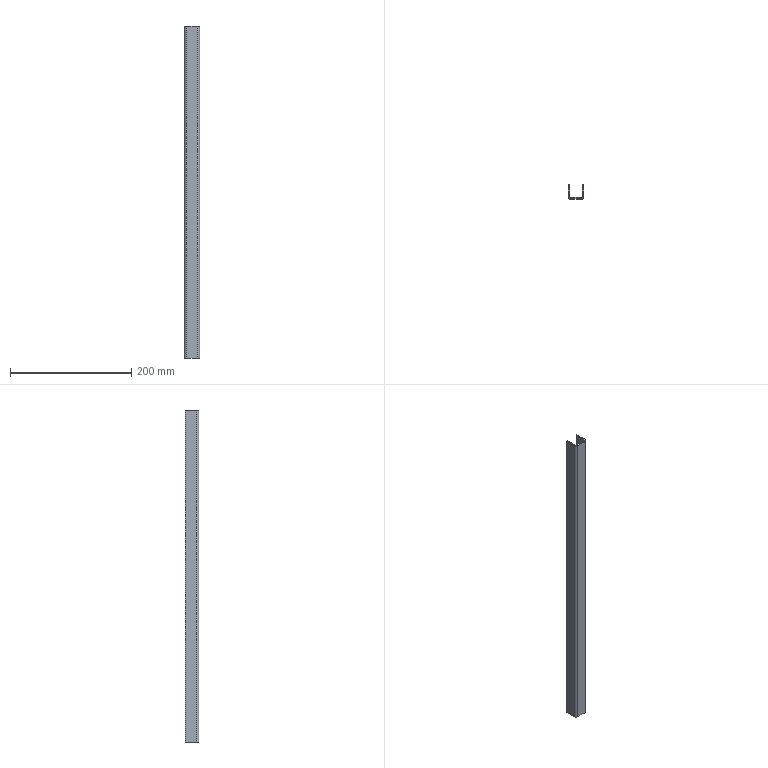Part | NX | features solid 2 | 1 solid | 14 faces | box 25 x 23 x 547 mm | volume 70481 mm3 | plane 10 | cylinder 4 | commonest cylinder face diameters 4 x2 8 x2
STEP:
#1=CARTESIAN_POINT('',(1215.,-671.,1137.));
#2=VERTEX_POINT('',#1);
#3=CARTESIAN_POINT('',(1215.,-652.,1137.));
#4=VERTEX_POINT('',#3);
#5=CARTESIAN_POINT('',(1215.,-652.,1137.));
#6=DIRECTION('',(0.,1.,0.));
#7=VECTOR('',#6,1000.);
#8=LINE('',#5,#7);
#9=EDGE_CURVE('',#2,#4,#8,.T.);
#10=ORIENTED_EDGE('',*,*,#9,.T.);
#11=CARTESIAN_POINT('',(1215.,-652.,590.));
#12=VERTEX_POINT('',#11);
#13=CARTESIAN_POINT('',(1215.,-652.,590.));
#14=DIRECTION('',(0.,0.,1.));
#15=VECTOR('',#14,1000.);
#16=LINE('',#13,#15);
#17=EDGE_CURVE('',#12,#4,#16,.T.);
#18=ORIENTED_EDGE('',*,*,#17,.F.);
#19=CARTESIAN_POINT('',(1215.,-671.,590.));
#20=VERTEX_POINT('',#19);
#21=CARTESIAN_POINT('',(1215.,-652.,590.));
#22=DIRECTION('',(0.,1.,0.));
#23=VECTOR('',#22,1000.);
#24=LINE('',#21,#23);
#25=EDGE_CURVE('',#20,#12,#24,.T.);
#26=ORIENTED_EDGE('',*,*,#25,.F.);
#27=CARTESIAN_POINT('',(1215.,-671.,590.));
#28=DIRECTION('',(0.,0.,1.));
#29=VECTOR('',#28,1000.);
#30=LINE('',#27,#29);
#31=EDGE_CURVE('',#20,#2,#30,.T.);
#32=ORIENTED_EDGE('',*,*,#31,.T.);
#33=EDGE_LOOP('',(#10,#18,#26,#32));
#34=FACE_BOUND('',#33,.T.);
#35=CARTESIAN_POINT('',(1215.,-652.,590.));
#36=DIRECTION('',(1.,0.,0.));
#37=DIRECTION('',(0.,0.,1.));
#38=AXIS2_PLACEMENT_3D('',#35,#36,#37);
#39=PLANE('',#38);
#40=ADVANCED_FACE('',(#34),#39,.F.);
#41=CARTESIAN_POINT('',(1219.,-675.,1137.));
#42=VERTEX_POINT('',#41);
#43=CARTESIAN_POINT('',(1219.,-671.,1137.));
#44=DIRECTION('',(0.,0.,-1.));
#45=DIRECTION('',(0.,-1.,0.));
#46=AXIS2_PLACEMENT_3D('',#43,#44,#45);
#47=CIRCLE('',#46,4.);
#48=EDGE_CURVE('',#42,#2,#47,.T.);
#49=ORIENTED_EDGE('',*,*,#48,.T.);
#50=ORIENTED_EDGE('',*,*,#31,.F.);
#51=CARTESIAN_POINT('',(1219.,-675.,590.));
#52=VERTEX_POINT('',#51);
#53=CARTESIAN_POINT('',(1219.,-671.,590.));
#54=DIRECTION('',(0.,0.,-1.));
#55=DIRECTION('',(0.,-1.,0.));
#56=AXIS2_PLACEMENT_3D('',#53,#54,#55);
#57=CIRCLE('',#56,4.);
#58=EDGE_CURVE('',#52,#20,#57,.T.);
#59=ORIENTED_EDGE('',*,*,#58,.F.);
#60=CARTESIAN_POINT('',(1219.,-675.,590.));
#61=DIRECTION('',(0.,0.,1.));
#62=VECTOR('',#61,1000.);
#63=LINE('',#60,#62);
#64=EDGE_CURVE('',#52,#42,#63,.T.);
#65=ORIENTED_EDGE('',*,*,#64,.T.);
#66=EDGE_LOOP('',(#49,#50,#59,#65));
#67=FACE_BOUND('',#66,.T.);
#68=CARTESIAN_POINT('',(1219.,-671.,590.));
#69=DIRECTION('',(0.,0.,1.));
#70=DIRECTION('',(0.,-1.,0.));
#71=AXIS2_PLACEMENT_3D('',#68,#69,#70);
#72=CYLINDRICAL_SURFACE('',#71,4.);
#73=ADVANCED_FACE('',(#67),#72,.T.);
#74=CARTESIAN_POINT('',(1236.,-675.,1137.));
#75=VERTEX_POINT('',#74);
#76=CARTESIAN_POINT('',(1217.,-675.,1137.));
#77=DIRECTION('',(-1.,0.,0.));
#78=VECTOR('',#77,1000.);
#79=LINE('',#76,#78);
#80=EDGE_CURVE('',#75,#42,#79,.T.);
#81=ORIENTED_EDGE('',*,*,#80,.T.);
#82=ORIENTED_EDGE('',*,*,#64,.F.);
#83=CARTESIAN_POINT('',(1236.,-675.,590.));
#84=VERTEX_POINT('',#83);
#85=CARTESIAN_POINT('',(1217.,-675.,590.));
#86=DIRECTION('',(-1.,0.,0.));
#87=VECTOR('',#86,1000.);
#88=LINE('',#85,#87);
#89=EDGE_CURVE('',#84,#52,#88,.T.);
#90=ORIENTED_EDGE('',*,*,#89,.F.);
#91=CARTESIAN_POINT('',(1236.,-675.,590.));
#92=DIRECTION('',(0.,0.,1.));
#93=VECTOR('',#92,1000.);
#94=LINE('',#91,#93);
#95=EDGE_CURVE('',#84,#75,#94,.T.);
#96=ORIENTED_EDGE('',*,*,#95,.T.);
#97=EDGE_LOOP('',(#81,#82,#90,#96));
#98=FACE_BOUND('',#97,.T.);
#99=CARTESIAN_POINT('',(1217.,-675.,590.));
#100=DIRECTION('',(0.,1.,0.));
#101=DIRECTION('',(0.,0.,-1.));
#102=AXIS2_PLACEMENT_3D('',#99,#100,#101);
#103=PLANE('',#102);
#104=ADVANCED_FACE('',(#98),#103,.F.);
#105=CARTESIAN_POINT('',(1240.,-671.,1137.));
#106=VERTEX_POINT('',#105);
#107=CARTESIAN_POINT('',(1236.,-671.,1137.));
#108=DIRECTION('',(0.,0.,-1.));
#109=DIRECTION('',(0.,-1.,0.));
#110=AXIS2_PLACEMENT_3D('',#107,#108,#109);
#111=CIRCLE('',#110,4.);
#112=EDGE_CURVE('',#106,#75,#111,.T.);
#113=ORIENTED_EDGE('',*,*,#112,.T.);
#114=ORIENTED_EDGE('',*,*,#95,.F.);
#115=CARTESIAN_POINT('',(1240.,-671.,590.));
#116=VERTEX_POINT('',#115);
#117=CARTESIAN_POINT('',(1236.,-671.,590.));
#118=DIRECTION('',(0.,0.,-1.));
#119=DIRECTION('',(0.,-1.,0.));
#120=AXIS2_PLACEMENT_3D('',#117,#118,#119);
#121=CIRCLE('',#120,4.);
#122=EDGE_CURVE('',#116,#84,#121,.T.);
#123=ORIENTED_EDGE('',*,*,#122,.F.);
#124=CARTESIAN_POINT('',(1240.,-671.,590.));
#125=DIRECTION('',(0.,0.,1.));
#126=VECTOR('',#125,1000.);
#127=LINE('',#124,#126);
#128=EDGE_CURVE('',#116,#106,#127,.T.);
#129=ORIENTED_EDGE('',*,*,#128,.T.);
#130=EDGE_LOOP('',(#113,#114,#123,#129));
#131=FACE_BOUND('',#130,.T.);
#132=CARTESIAN_POINT('',(1236.,-671.,590.));
#133=DIRECTION('',(0.,0.,1.));
#134=DIRECTION('',(0.,-1.,0.));
#135=AXIS2_PLACEMENT_3D('',#132,#133,#134);
#136=CYLINDRICAL_SURFACE('',#135,4.);
#137=ADVANCED_FACE('',(#131),#136,.T.);
#138=CARTESIAN_POINT('',(1240.,-652.,1137.));
#139=VERTEX_POINT('',#138);
#140=CARTESIAN_POINT('',(1240.,-673.,1137.));
#141=DIRECTION('',(0.,-1.,0.));
#142=VECTOR('',#141,1000.);
#143=LINE('',#140,#142);
#144=EDGE_CURVE('',#139,#106,#143,.T.);
#145=ORIENTED_EDGE('',*,*,#144,.T.);
#146=ORIENTED_EDGE('',*,*,#128,.F.);
#147=CARTESIAN_POINT('',(1240.,-652.,590.));
#148=VERTEX_POINT('',#147);
#149=CARTESIAN_POINT('',(1240.,-673.,590.));
#150=DIRECTION('',(0.,-1.,0.));
#151=VECTOR('',#150,1000.);
#152=LINE('',#149,#151);
#153=EDGE_CURVE('',#148,#116,#152,.T.);
#154=ORIENTED_EDGE('',*,*,#153,.F.);
#155=CARTESIAN_POINT('',(1240.,-652.,590.));
#156=DIRECTION('',(0.,0.,1.));
#157=VECTOR('',#156,1000.);
#158=LINE('',#155,#157);
#159=EDGE_CURVE('',#148,#139,#158,.T.);
#160=ORIENTED_EDGE('',*,*,#159,.T.);
#161=EDGE_LOOP('',(#145,#146,#154,#160));
#162=FACE_BOUND('',#161,.T.);
#163=CARTESIAN_POINT('',(1240.,-673.,590.));
#164=DIRECTION('',(-1.,0.,0.));
#165=DIRECTION('',(0.,0.,1.));
#166=AXIS2_PLACEMENT_3D('',#163,#164,#165);
#167=PLANE('',#166);
#168=ADVANCED_FACE('',(#162),#167,.F.);
#169=CARTESIAN_POINT('',(1217.,-671.,1137.));
#170=VERTEX_POINT('',#169);
#171=CARTESIAN_POINT('',(1217.,-652.,1137.));
#172=VERTEX_POINT('',#171);
#173=CARTESIAN_POINT('',(1217.,-652.,1137.));
#174=DIRECTION('',(0.,1.,0.));
#175=VECTOR('',#174,1000.);
#176=LINE('',#173,#175);
#177=EDGE_CURVE('',#170,#172,#176,.T.);
#178=ORIENTED_EDGE('',*,*,#177,.F.);
#179=CARTESIAN_POINT('',(1217.,-671.,590.));
#180=VERTEX_POINT('',#179);
#181=CARTESIAN_POINT('',(1217.,-671.,590.));
#182=DIRECTION('',(0.,0.,1.));
#183=VECTOR('',#182,1000.);
#184=LINE('',#181,#183);
#185=EDGE_CURVE('',#180,#170,#184,.T.);
#186=ORIENTED_EDGE('',*,*,#185,.F.);
#187=CARTESIAN_POINT('',(1217.,-652.,590.));
#188=VERTEX_POINT('',#187);
#189=CARTESIAN_POINT('',(1217.,-652.,590.));
#190=DIRECTION('',(0.,1.,0.));
#191=VECTOR('',#190,1000.);
#192=LINE('',#189,#191);
#193=EDGE_CURVE('',#180,#188,#192,.T.);
#194=ORIENTED_EDGE('',*,*,#193,.T.);
#195=CARTESIAN_POINT('',(1217.,-652.,590.));
#196=DIRECTION('',(0.,0.,1.));
#197=VECTOR('',#196,1000.);
#198=LINE('',#195,#197);
#199=EDGE_CURVE('',#188,#172,#198,.T.);
#200=ORIENTED_EDGE('',*,*,#199,.T.);
#201=EDGE_LOOP('',(#178,#186,#194,#200));
#202=FACE_BOUND('',#201,.T.);
#203=CARTESIAN_POINT('',(1217.,-652.,590.));
#204=DIRECTION('',(1.,0.,0.));
#205=DIRECTION('',(0.,0.,1.));
#206=AXIS2_PLACEMENT_3D('',#203,#204,#205);
#207=PLANE('',#206);
#208=ADVANCED_FACE('',(#202),#207,.T.);
#209=CARTESIAN_POINT('',(1219.,-673.,1137.));
#210=VERTEX_POINT('',#209);
#211=CARTESIAN_POINT('',(1219.,-671.,1137.));
#212=DIRECTION('',(0.,0.,-1.));
#213=DIRECTION('',(0.,-1.,0.));
#214=AXIS2_PLACEMENT_3D('',#211,#212,#213);
#215=CIRCLE('',#214,2.);
#216=EDGE_CURVE('',#210,#170,#215,.T.);
#217=ORIENTED_EDGE('',*,*,#216,.F.);
#218=CARTESIAN_POINT('',(1219.,-673.,590.));
#219=VERTEX_POINT('',#218);
#220=CARTESIAN_POINT('',(1219.,-673.,590.));
#221=DIRECTION('',(0.,0.,1.));
#222=VECTOR('',#221,1000.);
#223=LINE('',#220,#222);
#224=EDGE_CURVE('',#219,#210,#223,.T.);
#225=ORIENTED_EDGE('',*,*,#224,.F.);
#226=CARTESIAN_POINT('',(1219.,-671.,590.));
#227=DIRECTION('',(0.,0.,-1.));
#228=DIRECTION('',(0.,-1.,0.));
#229=AXIS2_PLACEMENT_3D('',#226,#227,#228);
#230=CIRCLE('',#229,2.);
#231=EDGE_CURVE('',#219,#180,#230,.T.);
#232=ORIENTED_EDGE('',*,*,#231,.T.);
#233=ORIENTED_EDGE('',*,*,#185,.T.);
#234=EDGE_LOOP('',(#217,#225,#232,#233));
#235=FACE_BOUND('',#234,.T.);
#236=CARTESIAN_POINT('',(1219.,-671.,590.));
#237=DIRECTION('',(0.,0.,1.));
#238=DIRECTION('',(0.,-1.,0.));
#239=AXIS2_PLACEMENT_3D('',#236,#237,#238);
#240=CYLINDRICAL_SURFACE('',#239,2.);
#241=ADVANCED_FACE('',(#235),#240,.F.);
#242=CARTESIAN_POINT('',(1236.,-673.,1137.));
#243=VERTEX_POINT('',#242);
#244=CARTESIAN_POINT('',(1217.,-673.,1137.));
#245=DIRECTION('',(-1.,0.,0.));
#246=VECTOR('',#245,1000.);
#247=LINE('',#244,#246);
#248=EDGE_CURVE('',#243,#210,#247,.T.);
#249=ORIENTED_EDGE('',*,*,#248,.F.);
#250=CARTESIAN_POINT('',(1236.,-673.,590.));
#251=VERTEX_POINT('',#250);
#252=CARTESIAN_POINT('',(1236.,-673.,590.));
#253=DIRECTION('',(0.,0.,1.));
#254=VECTOR('',#253,1000.);
#255=LINE('',#252,#254);
#256=EDGE_CURVE('',#251,#243,#255,.T.);
#257=ORIENTED_EDGE('',*,*,#256,.F.);
#258=CARTESIAN_POINT('',(1217.,-673.,590.));
#259=DIRECTION('',(-1.,0.,0.));
#260=VECTOR('',#259,1000.);
#261=LINE('',#258,#260);
#262=EDGE_CURVE('',#251,#219,#261,.T.);
#263=ORIENTED_EDGE('',*,*,#262,.T.);
#264=ORIENTED_EDGE('',*,*,#224,.T.);
#265=EDGE_LOOP('',(#249,#257,#263,#264));
#266=FACE_BOUND('',#265,.T.);
#267=CARTESIAN_POINT('',(1217.,-673.,590.));
#268=DIRECTION('',(0.,1.,0.));
#269=DIRECTION('',(0.,0.,-1.));
#270=AXIS2_PLACEMENT_3D('',#267,#268,#269);
#271=PLANE('',#270);
#272=ADVANCED_FACE('',(#266),#271,.T.);
#273=CARTESIAN_POINT('',(1238.,-671.,1137.));
#274=VERTEX_POINT('',#273);
#275=CARTESIAN_POINT('',(1236.,-671.,1137.));
#276=DIRECTION('',(0.,0.,-1.));
#277=DIRECTION('',(0.,-1.,0.));
#278=AXIS2_PLACEMENT_3D('',#275,#276,#277);
#279=CIRCLE('',#278,2.);
#280=EDGE_CURVE('',#274,#243,#279,.T.);
#281=ORIENTED_EDGE('',*,*,#280,.F.);
#282=CARTESIAN_POINT('',(1238.,-671.,590.));
#283=VERTEX_POINT('',#282);
#284=CARTESIAN_POINT('',(1238.,-671.,590.));
#285=DIRECTION('',(0.,0.,1.));
#286=VECTOR('',#285,1000.);
#287=LINE('',#284,#286);
#288=EDGE_CURVE('',#283,#274,#287,.T.);
#289=ORIENTED_EDGE('',*,*,#288,.F.);
#290=CARTESIAN_POINT('',(1236.,-671.,590.));
#291=DIRECTION('',(0.,0.,-1.));
#292=DIRECTION('',(0.,-1.,0.));
#293=AXIS2_PLACEMENT_3D('',#290,#291,#292);
#294=CIRCLE('',#293,2.);
#295=EDGE_CURVE('',#283,#251,#294,.T.);
#296=ORIENTED_EDGE('',*,*,#295,.T.);
#297=ORIENTED_EDGE('',*,*,#256,.T.);
#298=EDGE_LOOP('',(#281,#289,#296,#297));
#299=FACE_BOUND('',#298,.T.);
#300=CARTESIAN_POINT('',(1236.,-671.,590.));
#301=DIRECTION('',(0.,0.,1.));
#302=DIRECTION('',(0.,-1.,0.));
#303=AXIS2_PLACEMENT_3D('',#300,#301,#302);
#304=CYLINDRICAL_SURFACE('',#303,2.);
#305=ADVANCED_FACE('',(#299),#304,.F.);
#306=CARTESIAN_POINT('',(1238.,-652.,1137.));
#307=VERTEX_POINT('',#306);
#308=CARTESIAN_POINT('',(1238.,-673.,1137.));
#309=DIRECTION('',(0.,-1.,0.));
#310=VECTOR('',#309,1000.);
#311=LINE('',#308,#310);
#312=EDGE_CURVE('',#307,#274,#311,.T.);
#313=ORIENTED_EDGE('',*,*,#312,.F.);
#314=CARTESIAN_POINT('',(1238.,-652.,590.));
#315=VERTEX_POINT('',#314);
#316=CARTESIAN_POINT('',(1238.,-652.,590.));
#317=DIRECTION('',(0.,0.,1.));
#318=VECTOR('',#317,1000.);
#319=LINE('',#316,#318);
#320=EDGE_CURVE('',#315,#307,#319,.T.);
#321=ORIENTED_EDGE('',*,*,#320,.F.);
#322=CARTESIAN_POINT('',(1238.,-673.,590.));
#323=DIRECTION('',(0.,-1.,0.));
#324=VECTOR('',#323,1000.);
#325=LINE('',#322,#324);
#326=EDGE_CURVE('',#315,#283,#325,.T.);
#327=ORIENTED_EDGE('',*,*,#326,.T.);
#328=ORIENTED_EDGE('',*,*,#288,.T.);
#329=EDGE_LOOP('',(#313,#321,#327,#328));
#330=FACE_BOUND('',#329,.T.);
#331=CARTESIAN_POINT('',(1238.,-673.,590.));
#332=DIRECTION('',(-1.,0.,0.));
#333=DIRECTION('',(0.,0.,1.));
#334=AXIS2_PLACEMENT_3D('',#331,#332,#333);
#335=PLANE('',#334);
#336=ADVANCED_FACE('',(#330),#335,.T.);
#337=ORIENTED_EDGE('',*,*,#159,.F.);
#338=CARTESIAN_POINT('',(1238.,-652.,590.));
#339=DIRECTION('',(-1.,0.,0.));
#340=VECTOR('',#339,1000.);
#341=LINE('',#338,#340);
#342=EDGE_CURVE('',#148,#315,#341,.T.);
#343=ORIENTED_EDGE('',*,*,#342,.T.);
#344=ORIENTED_EDGE('',*,*,#320,.T.);
#345=CARTESIAN_POINT('',(1238.,-652.,1137.));
#346=DIRECTION('',(-1.,0.,0.));
#347=VECTOR('',#346,1000.);
#348=LINE('',#345,#347);
#349=EDGE_CURVE('',#139,#307,#348,.T.);
#350=ORIENTED_EDGE('',*,*,#349,.F.);
#351=EDGE_LOOP('',(#337,#343,#344,#350));
#352=FACE_BOUND('',#351,.T.);
#353=CARTESIAN_POINT('',(1238.,-652.,590.));
#354=DIRECTION('',(0.,-1.,0.));
#355=DIRECTION('',(-1.,0.,0.));
#356=AXIS2_PLACEMENT_3D('',#353,#354,#355);
#357=PLANE('',#356);
#358=ADVANCED_FACE('',(#352),#357,.F.);
#359=ORIENTED_EDGE('',*,*,#312,.T.);
#360=ORIENTED_EDGE('',*,*,#280,.T.);
#361=ORIENTED_EDGE('',*,*,#248,.T.);
#362=ORIENTED_EDGE('',*,*,#216,.T.);
#363=ORIENTED_EDGE('',*,*,#177,.T.);
#364=CARTESIAN_POINT('',(1217.,-652.,1137.));
#365=DIRECTION('',(1.,0.,0.));
#366=VECTOR('',#365,1000.);
#367=LINE('',#364,#366);
#368=EDGE_CURVE('',#4,#172,#367,.T.);
#369=ORIENTED_EDGE('',*,*,#368,.F.);
#370=ORIENTED_EDGE('',*,*,#9,.F.);
#371=ORIENTED_EDGE('',*,*,#48,.F.);
#372=ORIENTED_EDGE('',*,*,#80,.F.);
#373=ORIENTED_EDGE('',*,*,#112,.F.);
#374=ORIENTED_EDGE('',*,*,#144,.F.);
#375=ORIENTED_EDGE('',*,*,#349,.T.);
#376=EDGE_LOOP('',(#359,#360,#361,#362,#363,#369,#370,#371,#372,#373,#374,#375));
#377=FACE_BOUND('',#376,.T.);
#378=CARTESIAN_POINT('',(1238.,-673.,1137.));
#379=DIRECTION('',(0.,0.,-1.));
#380=DIRECTION('',(0.,-1.,0.));
#381=AXIS2_PLACEMENT_3D('',#378,#379,#380);
#382=PLANE('',#381);
#383=ADVANCED_FACE('',(#377),#382,.F.);
#384=CARTESIAN_POINT('',(1217.,-652.,590.));
#385=DIRECTION('',(1.,0.,0.));
#386=VECTOR('',#385,1000.);
#387=LINE('',#384,#386);
#388=EDGE_CURVE('',#12,#188,#387,.T.);
#389=ORIENTED_EDGE('',*,*,#388,.F.);
#390=ORIENTED_EDGE('',*,*,#17,.T.);
#391=ORIENTED_EDGE('',*,*,#368,.T.);
#392=ORIENTED_EDGE('',*,*,#199,.F.);
#393=EDGE_LOOP('',(#389,#390,#391,#392));
#394=FACE_BOUND('',#393,.T.);
#395=CARTESIAN_POINT('',(1217.,-652.,590.));
#396=DIRECTION('',(0.,1.,0.));
#397=DIRECTION('',(0.,0.,-1.));
#398=AXIS2_PLACEMENT_3D('',#395,#396,#397);
#399=PLANE('',#398);
#400=ADVANCED_FACE('',(#394),#399,.T.);
#401=ORIENTED_EDGE('',*,*,#193,.F.);
#402=ORIENTED_EDGE('',*,*,#231,.F.);
#403=ORIENTED_EDGE('',*,*,#262,.F.);
#404=ORIENTED_EDGE('',*,*,#295,.F.);
#405=ORIENTED_EDGE('',*,*,#326,.F.);
#406=ORIENTED_EDGE('',*,*,#342,.F.);
#407=ORIENTED_EDGE('',*,*,#153,.T.);
#408=ORIENTED_EDGE('',*,*,#122,.T.);
#409=ORIENTED_EDGE('',*,*,#89,.T.);
#410=ORIENTED_EDGE('',*,*,#58,.T.);
#411=ORIENTED_EDGE('',*,*,#25,.T.);
#412=ORIENTED_EDGE('',*,*,#388,.T.);
#413=EDGE_LOOP('',(#401,#402,#403,#404,#405,#406,#407,#408,#409,#410,#411,#412));
#414=FACE_BOUND('',#413,.T.);
#415=CARTESIAN_POINT('',(1217.,-652.,590.));
#416=DIRECTION('',(0.,0.,-1.));
#417=DIRECTION('',(0.,-1.,0.));
#418=AXIS2_PLACEMENT_3D('',#415,#416,#417);
#419=PLANE('',#418);
#420=ADVANCED_FACE('',(#414),#419,.T.);
#421=CLOSED_SHELL('',(#40,#73,#104,#137,#168,#208,#241,#272,#305,#336,#358,#383,#400,#420));
#422=MANIFOLD_SOLID_BREP('',#421);
#423=(LENGTH_UNIT()NAMED_UNIT(*)SI_UNIT(.MILLI.,.METRE.));
#424=UNCERTAINTY_MEASURE_WITH_UNIT(LENGTH_MEASURE(0.00001),#423,'','');
#425=(NAMED_UNIT(*)PLANE_ANGLE_UNIT()SI_UNIT($,.RADIAN.));
#426=(NAMED_UNIT(*)SI_UNIT($,.STERADIAN.)SOLID_ANGLE_UNIT());
#427=(GEOMETRIC_REPRESENTATION_CONTEXT(3)GLOBAL_UNCERTAINTY_ASSIGNED_CONTEXT((#424))GLOBAL_UNIT_ASSIGNED_CONTEXT((#423,#425,#426))REPRESENTATION_CONTEXT('',''));
#428=ADVANCED_BREP_SHAPE_REPRESENTATION('',(#422),#427);